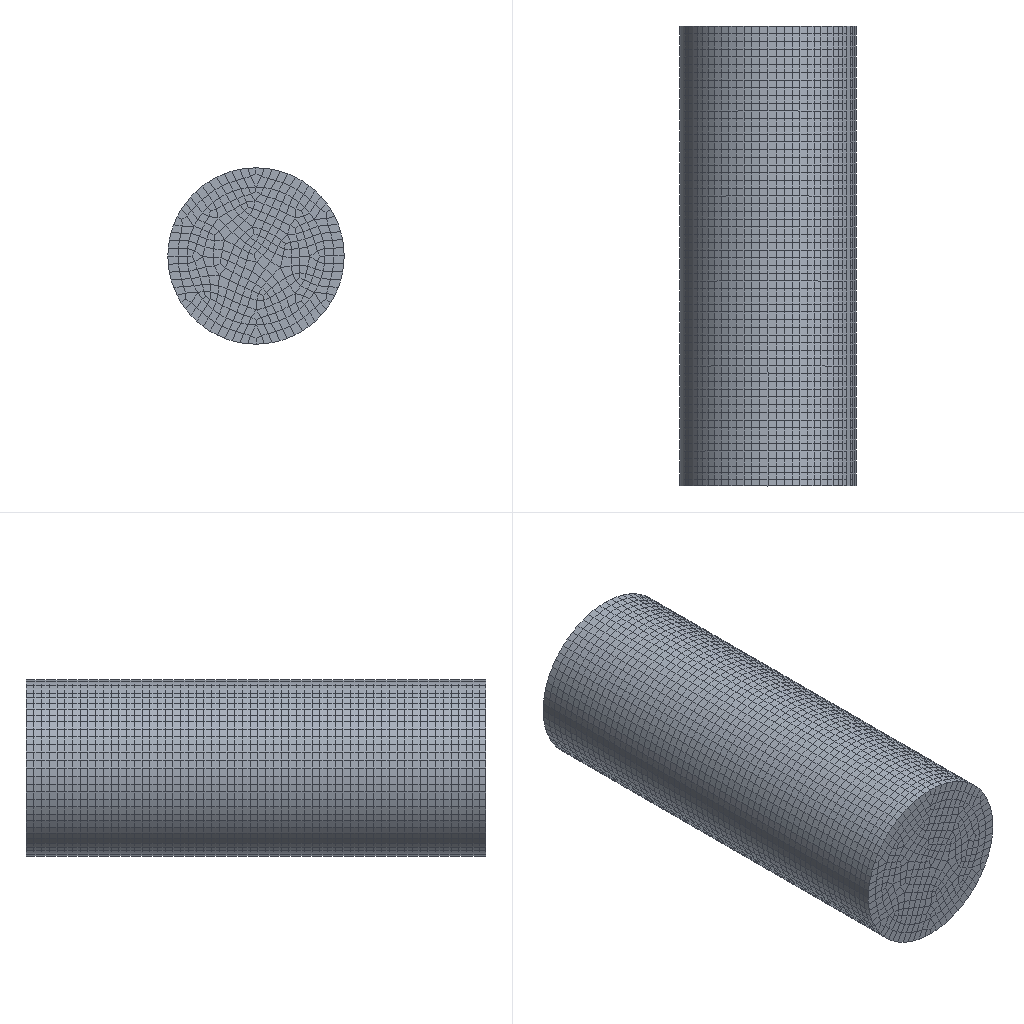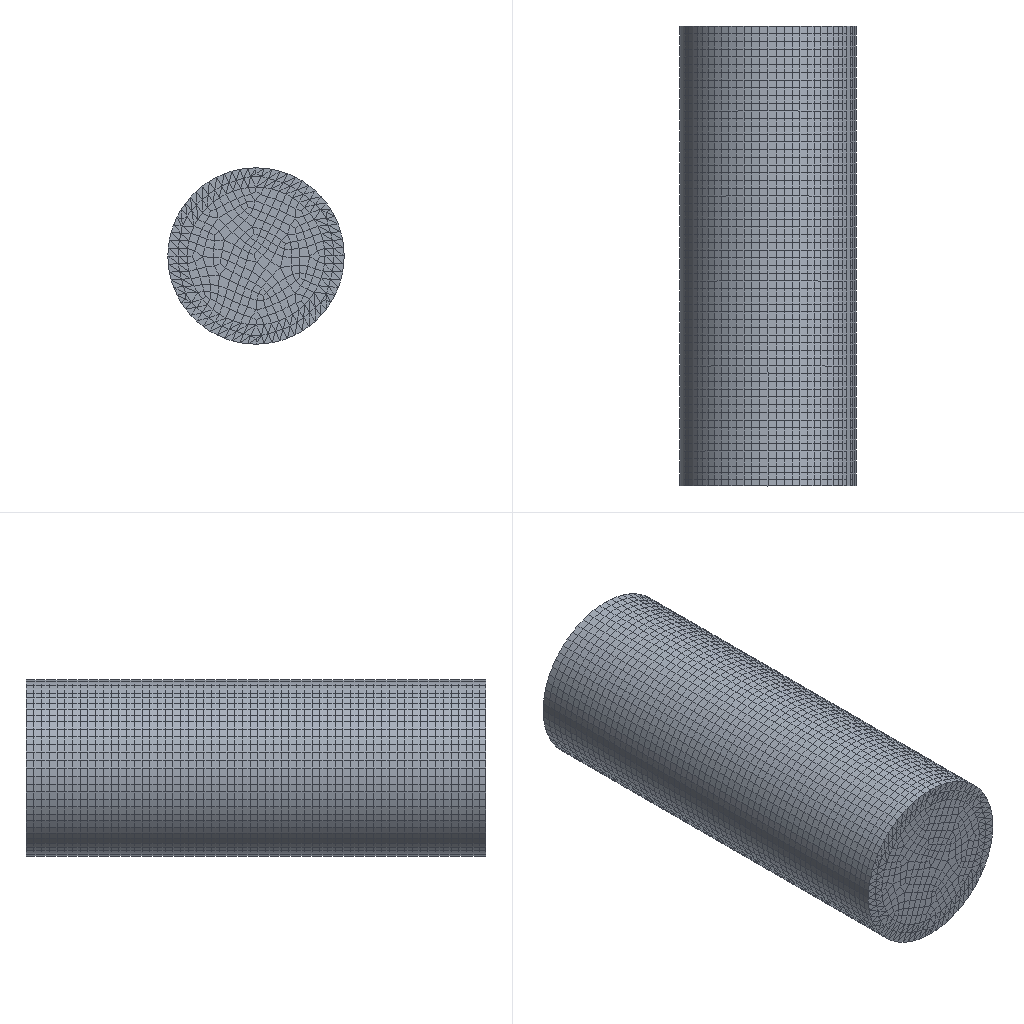Simulation study | ansys workbench
Set-up summary:
category,name,step,type,value,unit,region
solver,ansys_workbench
units,mm-N-s-tonne (MPa),,stated,"/units,MPA"
analysis,deck-1/LS1,,steady-state thermal
load_step,deck-1/LS1,deck-1/LS1,steady-state thermal,nsubst=1; time=1
analysis,deck-2/LS1,,static
load_step,deck-2/LS1,deck-2/LS1,static,nsubst=1; time=1
mesh,deck-1.dat,,nodes,46128
mesh,deck-1.dat,,elements,12591
element_type,SOLID90,,,8511,,deck-1.dat
element_type,SURF152,,,4080,,deck-1.dat
mesh,deck-2.dat,,nodes,46129
mesh,deck-2.dat,,elements,8878
element_type,SOLID186,,,8511,,deck-2.dat
element_type,CONTA174,,,367,,deck-2.dat
material,Structural Steel,,E,2e+11,Pa
material,Structural Steel,,nu,0.3
material,Structural Steel,,density,7850,kg m^-3
material,Structural Steel,,conductivity,60.5,W m^-1 C^-1
material,Structural Steel,,specific_heat,434,J kg^-1 C^-1
material,Structural Steel,,cte,1.2e-05,C^-1
material,Structural Steel,,permeability,10000
material,Structural Steel,,resistivity,1.7e-07,kg m^3 A^-2 s^-3
material,Structural Steel,,E,200000,tonne s^-2 mm^-1
material,Structural Steel,,nu,0.3
material,Structural Steel,,density,7.85e-09,tonne mm^-3
material,Structural Steel,,conductivity,60.5,tonne mm s^-3 C^-1
material,Structural Steel,,specific_heat,4.34e+08,mm^2 s^-2 C^-1
material,Structural Steel,,cte,1.2e-05,C^-1
material,Structural Steel,,permeability,10000
material,Structural Steel,,resistivity,0.00017,ohm mm
load,Define Uniform Initial temperature,deck-1/model,body load temp,22,,all
load,"Create ""______""",deck-1/LS1,convection,250,,SURF152 #2
load,ACEL,deck-2/LS1,gravity (ACEL; gravity acts opposite),"9806.65 [dir=(0, -1, 0)]",,all
load,"Create Imported Load ""________""",deck-2/LS1,body load temp,100 [n=46128],,all
bc,,deck-1/LS1,temperature,100 [dofs=TEMP],,node list
bc,,deck-2/LS1,fixed,"[dofs=ROTX,ROTY,ROTZ,UX,UY,UZ n=6]",,node list
contact,contact 1,,bonded (always),element=CONTA174
named_set,_CM33,,node,10344
named_set,REMOTEDISPALL,,node,1
Results summary:
result,analyses[0].index,,,1
result,analyses[0].system,,,SYS
result,analyses[0].deck,,,deck-1.dat
result,analyses[0].solve_status,,,completed
result,analyses[0].analysis_type,,,static
result,analyses[0].physics,,,thermal
result,analyses[0].unit_system,,,"MKS: m, kg, N, s, V, A, degC"
result,analyses[0].n_sets,,,1
result,analyses[0].load_steps[0].set,set=1,,1
result,analyses[0].load_steps[0].time_or_freq,set=1,,1
result,analyses[0].load_steps[0].max_temperature,set=1,,100
result,analyses[0].load_steps[0].min_temperature,set=1,,97.697
result,analyses[1].index,,,2
result,analyses[1].system,,,SYS-1
result,analyses[1].deck,,,deck-2.dat
result,analyses[1].solve_status,,,completed
result,analyses[1].analysis_type,,,static
result,analyses[1].physics,,,mechanical
result,analyses[1].unit_system,,,"NMM: mm, ton, N, s, mV, mA, degC"
result,analyses[1].n_sets,,,1
result,analyses[1].load_steps[0].set,set=1,,1
result,analyses[1].load_steps[0].time_or_freq,set=1,,1
result,analyses[1].load_steps[0].max_displacement_magnitude,set=1,,0.1122
result,analyses[1].load_steps[0].max_von_mises_nodal,set=1,,4.467
result,analyses[1].load_steps[0].reaction_force_sum_xyz[1],set=1,,-0.4409
result,analyses[1].load_steps[0].reaction_force_sum_xyz[2],set=1,,6.188
result,analyses[1].load_steps[0].reaction_force_sum_xyz[3],set=1,,0.02483
result,geometry_export[0][0],,,.step
result,geometry_export[0][1],,,ok
result,geometry_export[0][2],,,1